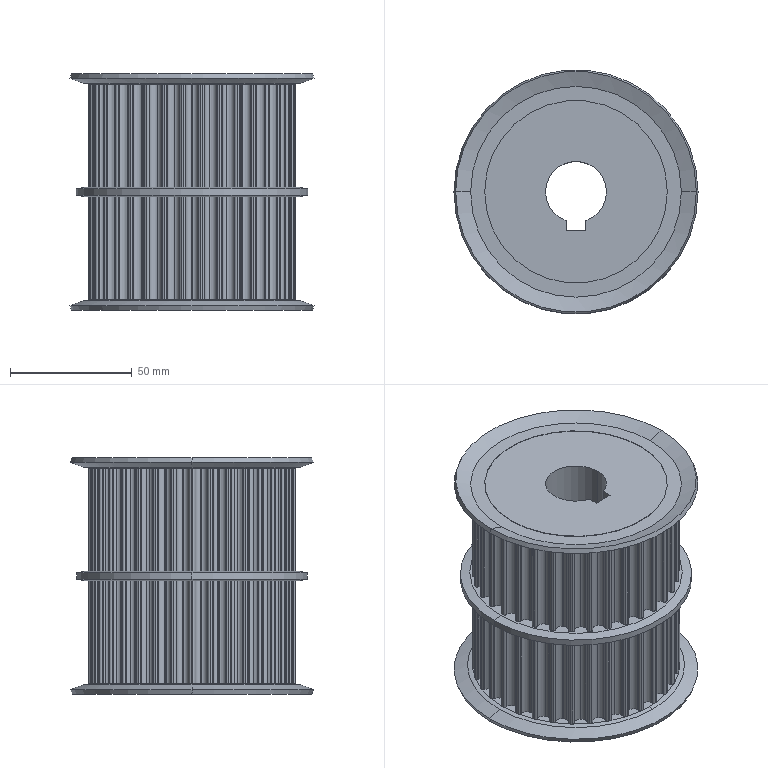Part | SolidWorks | features BaseBody 1 | 1 solid | 719 faces | box 100.208 x 100.208 x 97.168 mm | volume 413312 mm3 | cylinder 417 | plane 282 | cone 16 | spline 4 | commonest cylinder face diameters 1.6 x168 5.14 x168 85.208 x70 75 x4 25 x3 42 x2